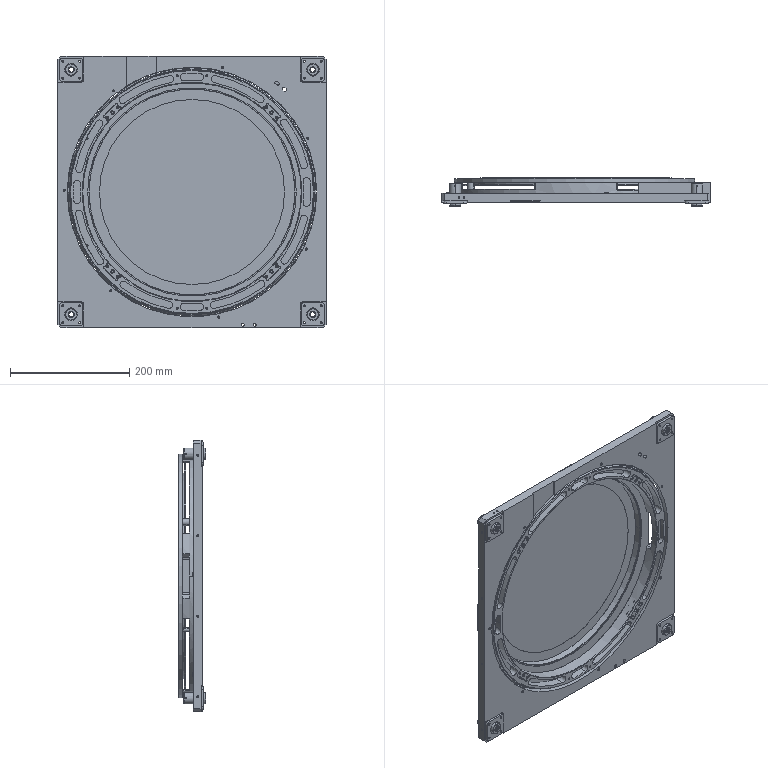Part | NX | features BREP 17 | 49 solids | 2076 faces | box 450 x 46.9 x 455 mm | volume 1668771 mm3 | cylinder 986 | plane 573 | cone 399 | torus 92 | spline 26 | commonest cylinder face diameters 4 x225 3.3 x102 10 x72 8.4 x52 6 x48 11 x42